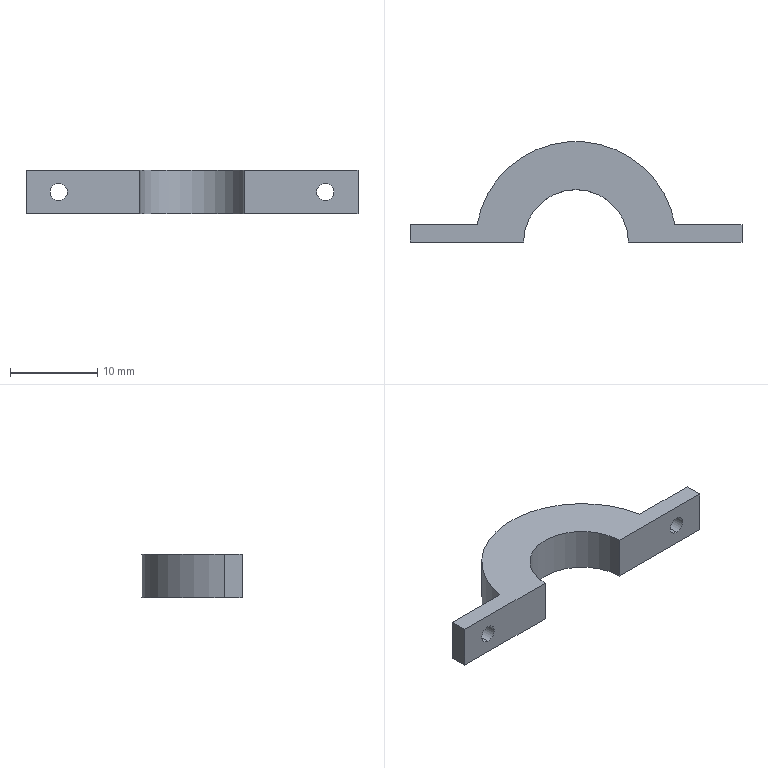Part | SolidWorks | features ICE 2, Extrusion 1 | 1 solid | 14 faces | box 38 x 11.5 x 5 mm | volume 894.544 mm3 | plane 8 | cylinder 6 | commonest cylinder face diameters 2 x4 12 x1 23 x1
STEP:
#1=CARTESIAN_POINT('',(-17.167,0.,1.5));
#2=VERTEX_POINT('',#1);
#3=CARTESIAN_POINT('',(-17.167,0.,3.5));
#4=VERTEX_POINT('',#3);
#5=CARTESIAN_POINT('',(-17.167,0.,2.5));
#6=DIRECTION('',(0.,1.,0.));
#7=DIRECTION('',(0.,0.,1.));
#8=AXIS2_PLACEMENT_3D('',#5,#6,#7);
#9=CIRCLE('',#8,1.);
#10=EDGE_CURVE('',#2,#4,#9,.T.);
#11=ORIENTED_EDGE('',*,*,#10,.F.);
#12=CARTESIAN_POINT('',(-17.167,2.,1.5));
#13=VERTEX_POINT('',#12);
#14=CARTESIAN_POINT('',(-17.167,-5.,1.5));
#15=DIRECTION('',(0.,1.,0.));
#16=VECTOR('',#15,1000.);
#17=LINE('',#14,#16);
#18=EDGE_CURVE('',#2,#13,#17,.T.);
#19=ORIENTED_EDGE('',*,*,#18,.T.);
#20=CARTESIAN_POINT('',(-17.167,2.,3.5));
#21=VERTEX_POINT('',#20);
#22=CARTESIAN_POINT('',(-17.167,2.,2.5));
#23=DIRECTION('',(0.,1.,0.));
#24=DIRECTION('',(0.,0.,1.));
#25=AXIS2_PLACEMENT_3D('',#22,#23,#24);
#26=CIRCLE('',#25,1.);
#27=EDGE_CURVE('',#13,#21,#26,.T.);
#28=ORIENTED_EDGE('',*,*,#27,.T.);
#29=CARTESIAN_POINT('',(-17.167,-5.,3.5));
#30=DIRECTION('',(0.,1.,0.));
#31=VECTOR('',#30,1000.);
#32=LINE('',#29,#31);
#33=EDGE_CURVE('',#4,#21,#32,.T.);
#34=ORIENTED_EDGE('',*,*,#33,.F.);
#35=EDGE_LOOP('',(#11,#19,#28,#34));
#36=FACE_OUTER_BOUND('',#35,.T.);
#37=CARTESIAN_POINT('',(-17.167,-5.,2.5));
#38=DIRECTION('',(0.,1.,0.));
#39=DIRECTION('',(0.,0.,1.));
#40=AXIS2_PLACEMENT_3D('',#37,#38,#39);
#41=CYLINDRICAL_SURFACE('',#40,1.);
#42=ADVANCED_FACE('',(#36),#41,.F.);
#43=CARTESIAN_POINT('',(13.333,0.,1.5));
#44=VERTEX_POINT('',#43);
#45=CARTESIAN_POINT('',(13.333,0.,3.5));
#46=VERTEX_POINT('',#45);
#47=CARTESIAN_POINT('',(13.333,0.,2.5));
#48=DIRECTION('',(0.,1.,0.));
#49=DIRECTION('',(0.,0.,1.));
#50=AXIS2_PLACEMENT_3D('',#47,#48,#49);
#51=CIRCLE('',#50,1.);
#52=EDGE_CURVE('',#44,#46,#51,.T.);
#53=ORIENTED_EDGE('',*,*,#52,.F.);
#54=CARTESIAN_POINT('',(13.333,2.,1.5));
#55=VERTEX_POINT('',#54);
#56=CARTESIAN_POINT('',(13.333,-5.,1.5));
#57=DIRECTION('',(0.,1.,0.));
#58=VECTOR('',#57,1000.);
#59=LINE('',#56,#58);
#60=EDGE_CURVE('',#44,#55,#59,.T.);
#61=ORIENTED_EDGE('',*,*,#60,.T.);
#62=CARTESIAN_POINT('',(13.333,2.,3.5));
#63=VERTEX_POINT('',#62);
#64=CARTESIAN_POINT('',(13.333,2.,2.5));
#65=DIRECTION('',(0.,1.,0.));
#66=DIRECTION('',(0.,0.,-1.));
#67=AXIS2_PLACEMENT_3D('',#64,#65,#66);
#68=CIRCLE('',#67,1.);
#69=EDGE_CURVE('',#55,#63,#68,.T.);
#70=ORIENTED_EDGE('',*,*,#69,.T.);
#71=CARTESIAN_POINT('',(13.333,-5.,3.5));
#72=DIRECTION('',(0.,1.,0.));
#73=VECTOR('',#72,1000.);
#74=LINE('',#71,#73);
#75=EDGE_CURVE('',#46,#63,#74,.T.);
#76=ORIENTED_EDGE('',*,*,#75,.F.);
#77=EDGE_LOOP('',(#53,#61,#70,#76));
#78=FACE_OUTER_BOUND('',#77,.T.);
#79=CARTESIAN_POINT('',(13.333,-5.,2.5));
#80=DIRECTION('',(0.,1.,0.));
#81=DIRECTION('',(0.,0.,1.));
#82=AXIS2_PLACEMENT_3D('',#79,#80,#81);
#83=CYLINDRICAL_SURFACE('',#82,1.);
#84=ADVANCED_FACE('',(#78),#83,.F.);
#85=CARTESIAN_POINT('',(-17.167,0.,2.5));
#86=DIRECTION('',(0.,1.,0.));
#87=DIRECTION('',(0.,0.,1.));
#88=AXIS2_PLACEMENT_3D('',#85,#86,#87);
#89=CIRCLE('',#88,1.);
#90=EDGE_CURVE('',#4,#2,#89,.T.);
#91=ORIENTED_EDGE('',*,*,#90,.T.);
#92=ORIENTED_EDGE('',*,*,#10,.T.);
#93=EDGE_LOOP('',(#91,#92));
#94=FACE_BOUND('',#93,.T.);
#95=CARTESIAN_POINT('',(-20.917,0.,0.));
#96=VERTEX_POINT('',#95);
#97=CARTESIAN_POINT('',(-7.917,0.,0.));
#98=VERTEX_POINT('',#97);
#99=CARTESIAN_POINT('',(9.583,0.,0.));
#100=DIRECTION('',(1.,0.,0.));
#101=VECTOR('',#100,1000.);
#102=LINE('',#99,#101);
#103=EDGE_CURVE('',#96,#98,#102,.T.);
#104=ORIENTED_EDGE('',*,*,#103,.T.);
#105=CARTESIAN_POINT('',(-7.917,0.,5.));
#106=VERTEX_POINT('',#105);
#107=CARTESIAN_POINT('',(-7.917,0.,0.));
#108=DIRECTION('',(0.,0.,1.));
#109=VECTOR('',#108,1000.);
#110=LINE('',#107,#109);
#111=EDGE_CURVE('',#98,#106,#110,.T.);
#112=ORIENTED_EDGE('',*,*,#111,.T.);
#113=CARTESIAN_POINT('',(-20.917,0.,5.));
#114=VERTEX_POINT('',#113);
#115=CARTESIAN_POINT('',(-13.417,0.,5.));
#116=DIRECTION('',(1.,0.,0.));
#117=VECTOR('',#116,1000.);
#118=LINE('',#115,#117);
#119=EDGE_CURVE('',#114,#106,#118,.T.);
#120=ORIENTED_EDGE('',*,*,#119,.F.);
#121=CARTESIAN_POINT('',(-20.917,0.,5.));
#122=DIRECTION('',(0.,0.,-1.));
#123=VECTOR('',#122,1000.);
#124=LINE('',#121,#123);
#125=EDGE_CURVE('',#114,#96,#124,.T.);
#126=ORIENTED_EDGE('',*,*,#125,.T.);
#127=EDGE_LOOP('',(#104,#112,#120,#126));
#128=FACE_OUTER_BOUND('',#127,.T.);
#129=CARTESIAN_POINT('',(9.583,0.,5.));
#130=DIRECTION('',(0.,1.,0.));
#131=DIRECTION('',(0.,0.,1.));
#132=AXIS2_PLACEMENT_3D('',#129,#130,#131);
#133=PLANE('',#132);
#134=ADVANCED_FACE('',(#94,#128),#133,.F.);
#135=CARTESIAN_POINT('',(13.333,2.,2.5));
#136=DIRECTION('',(0.,1.,0.));
#137=DIRECTION('',(0.,0.,-1.));
#138=AXIS2_PLACEMENT_3D('',#135,#136,#137);
#139=CIRCLE('',#138,1.);
#140=EDGE_CURVE('',#63,#55,#139,.T.);
#141=ORIENTED_EDGE('',*,*,#140,.F.);
#142=ORIENTED_EDGE('',*,*,#69,.F.);
#143=EDGE_LOOP('',(#141,#142));
#144=FACE_BOUND('',#143,.T.);
#145=CARTESIAN_POINT('',(17.083,2.,0.));
#146=VERTEX_POINT('',#145);
#147=CARTESIAN_POINT('',(9.408,2.,0.));
#148=VERTEX_POINT('',#147);
#149=CARTESIAN_POINT('',(17.083,2.,0.));
#150=DIRECTION('',(-1.,0.,0.));
#151=VECTOR('',#150,1000.);
#152=LINE('',#149,#151);
#153=EDGE_CURVE('',#146,#148,#152,.T.);
#154=ORIENTED_EDGE('',*,*,#153,.T.);
#155=CARTESIAN_POINT('',(9.408,2.,5.));
#156=VERTEX_POINT('',#155);
#157=CARTESIAN_POINT('',(9.408,2.,5.));
#158=DIRECTION('',(0.,0.,-1.));
#159=VECTOR('',#158,1000.);
#160=LINE('',#157,#159);
#161=EDGE_CURVE('',#156,#148,#160,.T.);
#162=ORIENTED_EDGE('',*,*,#161,.F.);
#163=CARTESIAN_POINT('',(17.083,2.,5.));
#164=VERTEX_POINT('',#163);
#165=CARTESIAN_POINT('',(17.083,2.,5.));
#166=DIRECTION('',(-1.,0.,0.));
#167=VECTOR('',#166,1000.);
#168=LINE('',#165,#167);
#169=EDGE_CURVE('',#164,#156,#168,.T.);
#170=ORIENTED_EDGE('',*,*,#169,.F.);
#171=CARTESIAN_POINT('',(17.083,2.,5.));
#172=DIRECTION('',(0.,0.,-1.));
#173=VECTOR('',#172,1000.);
#174=LINE('',#171,#173);
#175=EDGE_CURVE('',#164,#146,#174,.T.);
#176=ORIENTED_EDGE('',*,*,#175,.T.);
#177=EDGE_LOOP('',(#154,#162,#170,#176));
#178=FACE_OUTER_BOUND('',#177,.T.);
#179=CARTESIAN_POINT('',(17.083,2.,5.));
#180=DIRECTION('',(0.,-1.,0.));
#181=DIRECTION('',(0.,0.,-1.));
#182=AXIS2_PLACEMENT_3D('',#179,#180,#181);
#183=PLANE('',#182);
#184=ADVANCED_FACE('',(#144,#178),#183,.F.);
#185=CARTESIAN_POINT('',(-13.242,2.,0.));
#186=VERTEX_POINT('',#185);
#187=CARTESIAN_POINT('',(-1.917,0.,0.));
#188=DIRECTION('',(0.,0.,1.));
#189=DIRECTION('',(1.,0.,0.));
#190=AXIS2_PLACEMENT_3D('',#187,#188,#189);
#191=CIRCLE('',#190,11.5);
#192=EDGE_CURVE('',#148,#186,#191,.T.);
#193=ORIENTED_EDGE('',*,*,#192,.T.);
#194=CARTESIAN_POINT('',(-13.242,2.,5.));
#195=VERTEX_POINT('',#194);
#196=CARTESIAN_POINT('',(-13.242,2.,5.));
#197=DIRECTION('',(0.,0.,-1.));
#198=VECTOR('',#197,1000.);
#199=LINE('',#196,#198);
#200=EDGE_CURVE('',#195,#186,#199,.T.);
#201=ORIENTED_EDGE('',*,*,#200,.F.);
#202=CARTESIAN_POINT('',(-1.917,0.,5.));
#203=DIRECTION('',(0.,0.,1.));
#204=DIRECTION('',(1.,0.,0.));
#205=AXIS2_PLACEMENT_3D('',#202,#203,#204);
#206=CIRCLE('',#205,11.5);
#207=EDGE_CURVE('',#156,#195,#206,.T.);
#208=ORIENTED_EDGE('',*,*,#207,.F.);
#209=ORIENTED_EDGE('',*,*,#161,.T.);
#210=EDGE_LOOP('',(#193,#201,#208,#209));
#211=FACE_OUTER_BOUND('',#210,.T.);
#212=CARTESIAN_POINT('',(-1.917,0.,5.));
#213=DIRECTION('',(0.,0.,-1.));
#214=DIRECTION('',(-1.,0.,0.));
#215=AXIS2_PLACEMENT_3D('',#212,#213,#214);
#216=CYLINDRICAL_SURFACE('',#215,11.5);
#217=ADVANCED_FACE('',(#211),#216,.T.);
#218=CARTESIAN_POINT('',(-17.167,2.,2.5));
#219=DIRECTION('',(0.,1.,0.));
#220=DIRECTION('',(0.,0.,1.));
#221=AXIS2_PLACEMENT_3D('',#218,#219,#220);
#222=CIRCLE('',#221,1.);
#223=EDGE_CURVE('',#21,#13,#222,.T.);
#224=ORIENTED_EDGE('',*,*,#223,.F.);
#225=ORIENTED_EDGE('',*,*,#27,.F.);
#226=EDGE_LOOP('',(#224,#225));
#227=FACE_BOUND('',#226,.T.);
#228=CARTESIAN_POINT('',(-20.917,2.,0.));
#229=VERTEX_POINT('',#228);
#230=CARTESIAN_POINT('',(-20.917,2.,0.));
#231=DIRECTION('',(-1.,0.,0.));
#232=VECTOR('',#231,1000.);
#233=LINE('',#230,#232);
#234=EDGE_CURVE('',#186,#229,#233,.T.);
#235=ORIENTED_EDGE('',*,*,#234,.T.);
#236=CARTESIAN_POINT('',(-20.917,2.,5.));
#237=VERTEX_POINT('',#236);
#238=CARTESIAN_POINT('',(-20.917,2.,5.));
#239=DIRECTION('',(0.,0.,-1.));
#240=VECTOR('',#239,1000.);
#241=LINE('',#238,#240);
#242=EDGE_CURVE('',#237,#229,#241,.T.);
#243=ORIENTED_EDGE('',*,*,#242,.F.);
#244=CARTESIAN_POINT('',(-20.917,2.,5.));
#245=DIRECTION('',(-1.,0.,0.));
#246=VECTOR('',#245,1000.);
#247=LINE('',#244,#246);
#248=EDGE_CURVE('',#195,#237,#247,.T.);
#249=ORIENTED_EDGE('',*,*,#248,.F.);
#250=ORIENTED_EDGE('',*,*,#200,.T.);
#251=EDGE_LOOP('',(#235,#243,#249,#250));
#252=FACE_OUTER_BOUND('',#251,.T.);
#253=CARTESIAN_POINT('',(-20.917,2.,5.));
#254=DIRECTION('',(0.,-1.,0.));
#255=DIRECTION('',(0.,0.,-1.));
#256=AXIS2_PLACEMENT_3D('',#253,#254,#255);
#257=PLANE('',#256);
#258=ADVANCED_FACE('',(#227,#252),#257,.F.);
#259=CARTESIAN_POINT('',(-20.917,0.,0.));
#260=DIRECTION('',(0.,-1.,0.));
#261=VECTOR('',#260,1000.);
#262=LINE('',#259,#261);
#263=EDGE_CURVE('',#229,#96,#262,.T.);
#264=ORIENTED_EDGE('',*,*,#263,.T.);
#265=ORIENTED_EDGE('',*,*,#125,.F.);
#266=CARTESIAN_POINT('',(-20.917,0.,5.));
#267=DIRECTION('',(0.,-1.,0.));
#268=VECTOR('',#267,1000.);
#269=LINE('',#266,#268);
#270=EDGE_CURVE('',#237,#114,#269,.T.);
#271=ORIENTED_EDGE('',*,*,#270,.F.);
#272=ORIENTED_EDGE('',*,*,#242,.T.);
#273=EDGE_LOOP('',(#264,#265,#271,#272));
#274=FACE_OUTER_BOUND('',#273,.T.);
#275=CARTESIAN_POINT('',(-20.917,0.,5.));
#276=DIRECTION('',(1.,0.,0.));
#277=DIRECTION('',(0.,0.,-1.));
#278=AXIS2_PLACEMENT_3D('',#275,#276,#277);
#279=PLANE('',#278);
#280=ADVANCED_FACE('',(#274),#279,.F.);
#281=CARTESIAN_POINT('',(13.333,0.,2.5));
#282=DIRECTION('',(0.,1.,0.));
#283=DIRECTION('',(0.,0.,1.));
#284=AXIS2_PLACEMENT_3D('',#281,#282,#283);
#285=CIRCLE('',#284,1.);
#286=EDGE_CURVE('',#46,#44,#285,.T.);
#287=ORIENTED_EDGE('',*,*,#286,.T.);
#288=ORIENTED_EDGE('',*,*,#52,.T.);
#289=EDGE_LOOP('',(#287,#288));
#290=FACE_BOUND('',#289,.T.);
#291=CARTESIAN_POINT('',(4.083,0.,5.));
#292=VERTEX_POINT('',#291);
#293=CARTESIAN_POINT('',(17.083,0.,5.));
#294=VERTEX_POINT('',#293);
#295=CARTESIAN_POINT('',(-13.417,0.,5.));
#296=DIRECTION('',(1.,0.,0.));
#297=VECTOR('',#296,1000.);
#298=LINE('',#295,#297);
#299=EDGE_CURVE('',#292,#294,#298,.T.);
#300=ORIENTED_EDGE('',*,*,#299,.F.);
#301=CARTESIAN_POINT('',(4.083,0.,0.));
#302=VERTEX_POINT('',#301);
#303=CARTESIAN_POINT('',(4.083,0.,0.));
#304=DIRECTION('',(0.,0.,-1.));
#305=VECTOR('',#304,1000.);
#306=LINE('',#303,#305);
#307=EDGE_CURVE('',#292,#302,#306,.T.);
#308=ORIENTED_EDGE('',*,*,#307,.T.);
#309=CARTESIAN_POINT('',(17.083,0.,0.));
#310=VERTEX_POINT('',#309);
#311=CARTESIAN_POINT('',(9.583,0.,0.));
#312=DIRECTION('',(1.,0.,0.));
#313=VECTOR('',#312,1000.);
#314=LINE('',#311,#313);
#315=EDGE_CURVE('',#302,#310,#314,.T.);
#316=ORIENTED_EDGE('',*,*,#315,.T.);
#317=CARTESIAN_POINT('',(17.083,0.,5.));
#318=DIRECTION('',(0.,0.,-1.));
#319=VECTOR('',#318,1000.);
#320=LINE('',#317,#319);
#321=EDGE_CURVE('',#294,#310,#320,.T.);
#322=ORIENTED_EDGE('',*,*,#321,.F.);
#323=EDGE_LOOP('',(#300,#308,#316,#322));
#324=FACE_OUTER_BOUND('',#323,.T.);
#325=CARTESIAN_POINT('',(9.583,0.,5.));
#326=DIRECTION('',(0.,1.,0.));
#327=DIRECTION('',(0.,0.,1.));
#328=AXIS2_PLACEMENT_3D('',#325,#326,#327);
#329=PLANE('',#328);
#330=ADVANCED_FACE('',(#290,#324),#329,.F.);
#331=CARTESIAN_POINT('',(17.083,0.,0.));
#332=DIRECTION('',(0.,1.,0.));
#333=VECTOR('',#332,1000.);
#334=LINE('',#331,#333);
#335=EDGE_CURVE('',#310,#146,#334,.T.);
#336=ORIENTED_EDGE('',*,*,#335,.T.);
#337=ORIENTED_EDGE('',*,*,#175,.F.);
#338=CARTESIAN_POINT('',(17.083,0.,5.));
#339=DIRECTION('',(0.,1.,0.));
#340=VECTOR('',#339,1000.);
#341=LINE('',#338,#340);
#342=EDGE_CURVE('',#294,#164,#341,.T.);
#343=ORIENTED_EDGE('',*,*,#342,.F.);
#344=ORIENTED_EDGE('',*,*,#321,.T.);
#345=EDGE_LOOP('',(#336,#337,#343,#344));
#346=FACE_OUTER_BOUND('',#345,.T.);
#347=CARTESIAN_POINT('',(17.083,0.,5.));
#348=DIRECTION('',(-1.,0.,0.));
#349=DIRECTION('',(0.,0.,1.));
#350=AXIS2_PLACEMENT_3D('',#347,#348,#349);
#351=PLANE('',#350);
#352=ADVANCED_FACE('',(#346),#351,.F.);
#353=CARTESIAN_POINT('',(-1.917,0.,5.));
#354=DIRECTION('',(0.,0.,1.));
#355=DIRECTION('',(1.,0.,0.));
#356=AXIS2_PLACEMENT_3D('',#353,#354,#355);
#357=CIRCLE('',#356,6.);
#358=EDGE_CURVE('',#292,#106,#357,.T.);
#359=ORIENTED_EDGE('',*,*,#358,.F.);
#360=ORIENTED_EDGE('',*,*,#299,.T.);
#361=ORIENTED_EDGE('',*,*,#342,.T.);
#362=ORIENTED_EDGE('',*,*,#169,.T.);
#363=ORIENTED_EDGE('',*,*,#207,.T.);
#364=ORIENTED_EDGE('',*,*,#248,.T.);
#365=ORIENTED_EDGE('',*,*,#270,.T.);
#366=ORIENTED_EDGE('',*,*,#119,.T.);
#367=EDGE_LOOP('',(#359,#360,#361,#362,#363,#364,#365,#366));
#368=FACE_OUTER_BOUND('',#367,.T.);
#369=CARTESIAN_POINT('',(-1.917,0.,5.));
#370=DIRECTION('',(0.,0.,1.));
#371=DIRECTION('',(1.,0.,0.));
#372=AXIS2_PLACEMENT_3D('',#369,#370,#371);
#373=PLANE('',#372);
#374=ADVANCED_FACE('',(#368),#373,.T.);
#375=ORIENTED_EDGE('',*,*,#315,.F.);
#376=CARTESIAN_POINT('',(-1.917,0.,0.));
#377=DIRECTION('',(0.,0.,1.));
#378=DIRECTION('',(1.,0.,0.));
#379=AXIS2_PLACEMENT_3D('',#376,#377,#378);
#380=CIRCLE('',#379,6.);
#381=EDGE_CURVE('',#302,#98,#380,.T.);
#382=ORIENTED_EDGE('',*,*,#381,.T.);
#383=ORIENTED_EDGE('',*,*,#103,.F.);
#384=ORIENTED_EDGE('',*,*,#263,.F.);
#385=ORIENTED_EDGE('',*,*,#234,.F.);
#386=ORIENTED_EDGE('',*,*,#192,.F.);
#387=ORIENTED_EDGE('',*,*,#153,.F.);
#388=ORIENTED_EDGE('',*,*,#335,.F.);
#389=EDGE_LOOP('',(#375,#382,#383,#384,#385,#386,#387,#388));
#390=FACE_OUTER_BOUND('',#389,.T.);
#391=CARTESIAN_POINT('',(-1.917,0.,0.));
#392=DIRECTION('',(0.,0.,1.));
#393=DIRECTION('',(1.,0.,0.));
#394=AXIS2_PLACEMENT_3D('',#391,#392,#393);
#395=PLANE('',#394);
#396=ADVANCED_FACE('',(#390),#395,.F.);
#397=ORIENTED_EDGE('',*,*,#60,.F.);
#398=ORIENTED_EDGE('',*,*,#286,.F.);
#399=ORIENTED_EDGE('',*,*,#75,.T.);
#400=ORIENTED_EDGE('',*,*,#140,.T.);
#401=EDGE_LOOP('',(#397,#398,#399,#400));
#402=FACE_OUTER_BOUND('',#401,.T.);
#403=CARTESIAN_POINT('',(13.333,-5.,2.5));
#404=DIRECTION('',(0.,1.,0.));
#405=DIRECTION('',(0.,0.,1.));
#406=AXIS2_PLACEMENT_3D('',#403,#404,#405);
#407=CYLINDRICAL_SURFACE('',#406,1.);
#408=ADVANCED_FACE('',(#402),#407,.F.);
#409=ORIENTED_EDGE('',*,*,#18,.F.);
#410=ORIENTED_EDGE('',*,*,#90,.F.);
#411=ORIENTED_EDGE('',*,*,#33,.T.);
#412=ORIENTED_EDGE('',*,*,#223,.T.);
#413=EDGE_LOOP('',(#409,#410,#411,#412));
#414=FACE_OUTER_BOUND('',#413,.T.);
#415=CARTESIAN_POINT('',(-17.167,-5.,2.5));
#416=DIRECTION('',(0.,1.,0.));
#417=DIRECTION('',(0.,0.,1.));
#418=AXIS2_PLACEMENT_3D('',#415,#416,#417);
#419=CYLINDRICAL_SURFACE('',#418,1.);
#420=ADVANCED_FACE('',(#414),#419,.F.);
#421=ORIENTED_EDGE('',*,*,#381,.F.);
#422=ORIENTED_EDGE('',*,*,#307,.F.);
#423=ORIENTED_EDGE('',*,*,#358,.T.);
#424=ORIENTED_EDGE('',*,*,#111,.F.);
#425=EDGE_LOOP('',(#421,#422,#423,#424));
#426=FACE_OUTER_BOUND('',#425,.T.);
#427=CARTESIAN_POINT('',(-1.917,0.,0.));
#428=DIRECTION('',(0.,0.,1.));
#429=DIRECTION('',(1.,0.,0.));
#430=AXIS2_PLACEMENT_3D('',#427,#428,#429);
#431=CYLINDRICAL_SURFACE('',#430,6.);
#432=ADVANCED_FACE('',(#426),#431,.F.);
#433=CLOSED_SHELL('',(#42,#84,#134,#184,#217,#258,#280,#330,#352,#374,#396,#408,#420,#432));
#434=MANIFOLD_SOLID_BREP('',#433);
#435=CARTESIAN_POINT('',(0.,0.,0.));
#436=DIRECTION('',(0.,0.,1.));
#437=DIRECTION('',(1.,0.,0.));
#438=AXIS2_PLACEMENT_3D('',#435,#436,#437);
#439=(LENGTH_UNIT()NAMED_UNIT(*)SI_UNIT(.MILLI.,.METRE.));
#440=UNCERTAINTY_MEASURE_WITH_UNIT(LENGTH_MEASURE(0.00001),#439,'','');
#441=(NAMED_UNIT(*)PLANE_ANGLE_UNIT()SI_UNIT($,.RADIAN.));
#442=(NAMED_UNIT(*)SI_UNIT($,.STERADIAN.)SOLID_ANGLE_UNIT());
#443=(GEOMETRIC_REPRESENTATION_CONTEXT(3)GLOBAL_UNCERTAINTY_ASSIGNED_CONTEXT((#440))GLOBAL_UNIT_ASSIGNED_CONTEXT((#439,#441,#442))REPRESENTATION_CONTEXT('',''));
#444=ADVANCED_BREP_SHAPE_REPRESENTATION('',(#434,#438),#443);